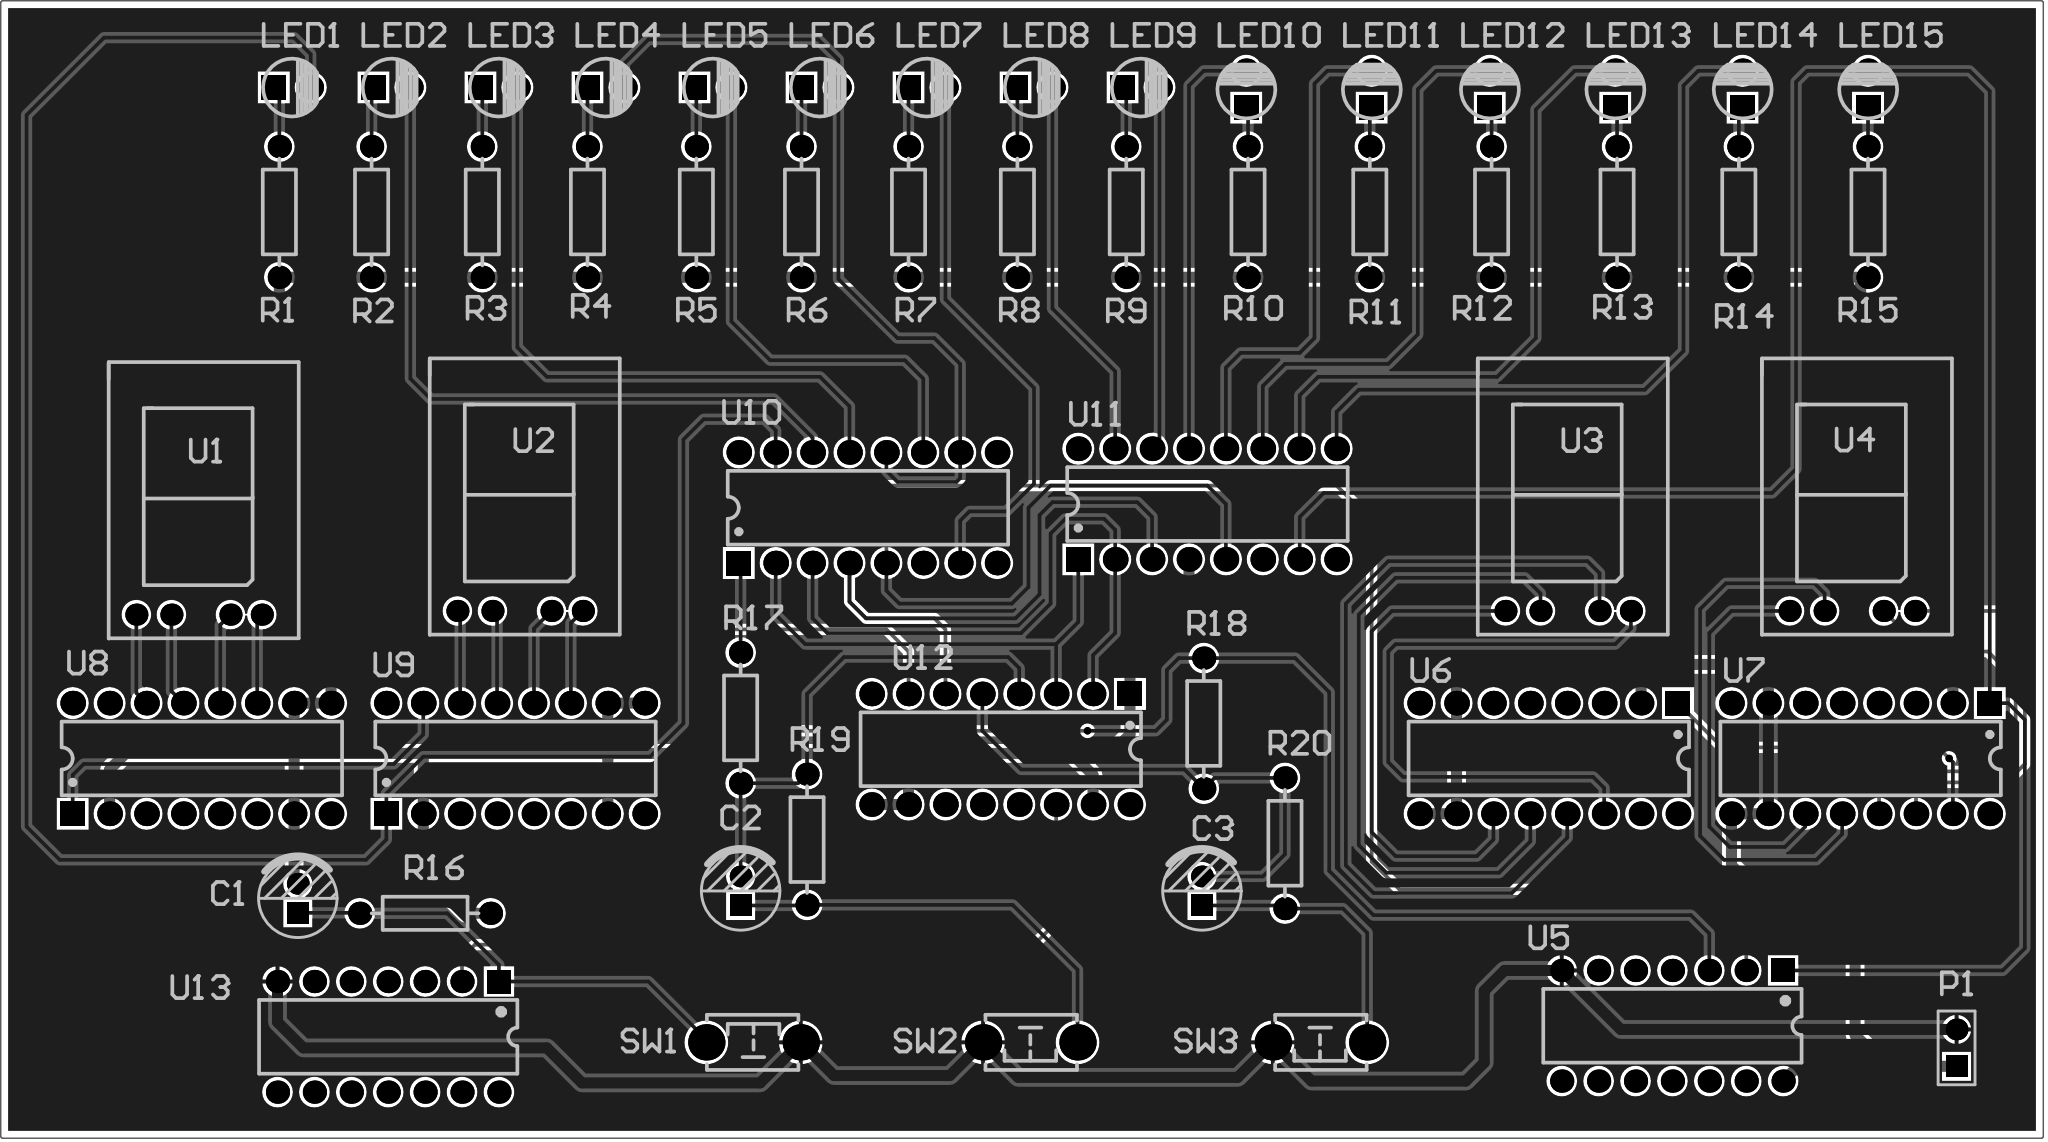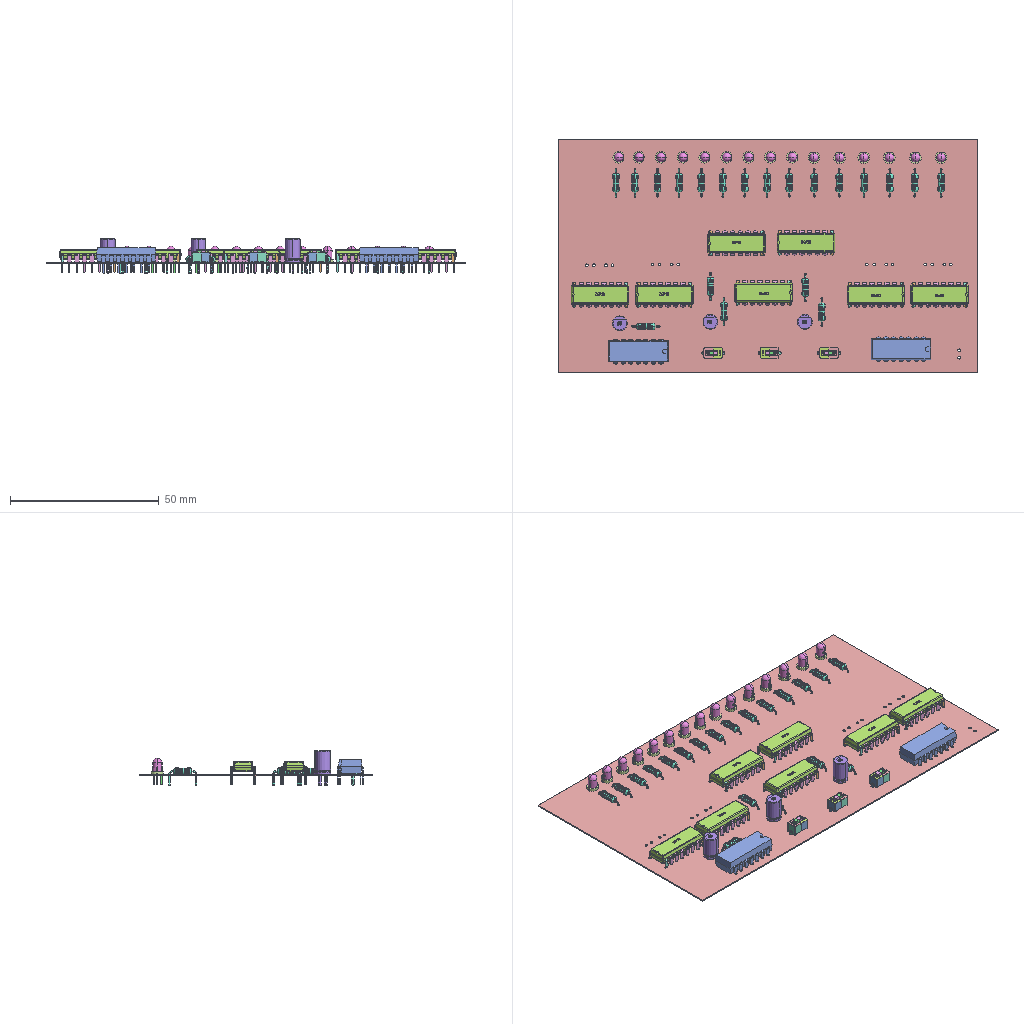Circuit board layout | Altium Designer | box 140.6 x 78.4 x 11.5 mm
Layer stack:
# Altium Designer layer stack of  (unit mm; dielectric type: 0 none, 1 core, 2 prepreg, 3 surface material)
index,name,kind,layer,copper_thickness_mm,dielectric_type,dielectric_thickness_mm,dielectric_material,dielectric_constant
0,Top Paste,other,,,,,,
1,Top Overlay,other,,,,,,
2,Top Solder,dielectric,,,3,0.0102,Solder Resist,3.5
3,Top Layer,copper,Top Layer,0.0356,,,,
4,Dielectric 1,dielectric,,,0,0.32,FR-4,4.8
5,Bottom Layer,copper,Bottom Layer,0.0356,,,,
6,Bottom Solder,dielectric,,,3,0.0102,Solder Resist,3.5
7,Bottom Overlay,other,,,,,,
8,Bottom Paste,other,,,,,,
# drill layer pairs: low layer,high layer
drill_pair,Top Layer,Bottom Layer
Part placement:
Designator,Comment,Layer,Footprint,Center-X(mm),Center-Y(mm),Rotation
U13,SN74LS04D,TopLayer,DIP14,55.118,48.768,270
U12,SN74LS193D,TopLayer,DIP16,97.282,68.58,270
SW3,3x6x5,TopLayer,TSW_DIP-3*6*4.3,119.253,48.387,180
SW2,3x6x5,TopLayer,TSW_DIP-3*6*4.3,99.314,48.387,180
SW1,3x6x5,TopLayer,TSW_DIP-3*6*4.3,80.264,48.387,360
C2,Cap,TopLayer,CS_2.0*5*8_-_C,79.375,58.817,270
C3,Cap,TopLayer,CS_2.0*5*8_-_C,111.125,58.817,270
C1,Cap,TopLayer,CS_2.0*5*8_-_C,48.895,58.309,270
LED1,LED1,TopLayer,LED_3MM-B,48.514,114.173,0
LED2,LED2,TopLayer,LED_3MM-B,55.372,114.173,0
LED3,LED3,TopLayer,LED_3MM-B,62.738,114.173,0
LED4,LED4,TopLayer,LED_3MM-B,70.104,114.173,0
LED5,LED1,TopLayer,LED_3MM-B,77.47,114.173,0
LED6,LED1,TopLayer,LED_3MM-B,84.836,114.173,0
LED7,LED1,TopLayer,LED_3MM-B,92.202,114.173,0
LED8,LED1,TopLayer,LED_3MM-B,99.568,114.173,0
LED9,LED1,TopLayer,LED_3MM-B,106.934,114.173,0
LED10,LED1,TopLayer,LED_3MM-B,114.173,114.046,90
LED11,LED1,TopLayer,LED_3MM-B,122.809,114.046,90
LED12,LED1,TopLayer,LED_3MM-B,130.937,114.046,90
LED13,LED1,TopLayer,LED_3MM-B,139.573,114.046,90
LED14,LED1,TopLayer,LED_3MM-B,148.336,114.046,90
LED15,LED1,TopLayer,LED_3MM-B,156.972,114.046,90
R1,,TopLayer,RS_1/4W,47.625,105.592,270
R2,Res1,TopLayer,RS_1/4W,53.975,105.592,270
R3,Res1,TopLayer,RS_1/4W,61.595,105.592,270
R4,Res1,TopLayer,RS_1/4W,68.834,105.592,270
R5,Res1,TopLayer,RS_1/4W,76.327,105.592,270
R6,Res1,TopLayer,RS_1/4W,83.566,105.592,270
R7,Res1,TopLayer,RS_1/4W,90.932,105.592,270
R8,Res1,TopLayer,RS_1/4W,98.425,105.592,270
R9,Res1,TopLayer,RS_1/4W,105.918,105.592,270
R10,Res1,TopLayer,RS_1/4W,114.3,105.592,270
R11,Res1,TopLayer,RS_1/4W,122.682,105.592,270
R12,Res1,TopLayer,RS_1/4W,131.064,105.592,270
R13,Res1,TopLayer,RS_1/4W,139.7,105.592,270
R14,Res1,TopLayer,RS_1/4W,148.082,105.592,270
R15,Res1,TopLayer,RS_1/4W,156.972,105.592,270
R17,Res1,TopLayer,RS_1/4W,79.375,70.739,90
R18,Res1,TopLayer,RS_1/4W,111.252,70.358,90
R19,Res1,TopLayer,RS_1/4W,83.947,62.357,90
R20,,TopLayer,RS_1/4W,116.84,62.103,90
R16,10k,TopLayer,RS_1/4W,57.658,57.277,360
U1,LCD1,TopLayer,DCD-HEX,42.1,77.851,360
U2,LCD1,TopLayer,DCD-HEX,64.198,78.105,0
U3,LCD1,TopLayer,DCD-HEX,136.334,78.105,0
U4,LCD1,TopLayer,DCD-HEX,155.893,78.105,0
U6,SN74LS160AD,TopLayer,DIP16,135.001,67.945,270
U7,SN74LS160AD,TopLayer,DIP16,156.464,67.945,270
U8,SN74LS160AD,TopLayer,DIP16,42.291,67.945,90
U9,SN74LS160AD,TopLayer,DIP16,63.881,67.945,90
U10,SN74LS138D,TopLayer,DIP16,88.138,85.217,90
U11,SN74LS138D,TopLayer,DIP16,111.506,85.471,90
U5,SN74LS08D,TopLayer,DIP14,143.51,49.53,270
P1,Header 2,TopLayer,HDR1X2,163.068,48.006,90
Pad and via stacks:
# Altium Designer via and pad stacks of  (unit mm). Each distinct definition once, with the count of objects using it.
# via: kind,start_layer,end_layer,hole_mm,diameter_mm,mode(0 simple;1 top-mid-bottom;2 full stack),diameter_per_layer,count,example_net
# pad: kind,layer,hole_mm,hole_type(0 round;1 square;2 slot),plating,top_size,top_shape(1 round;2 rect;3 octagon;9 rounded rect),mid_size,bottom_size,mode,footprint,size_per_layer,count,example
pad,Multi-Layer,0.8,0,plated,1.7x1.7,1,1.7x1.7,1.7x1.7,0,DIP16,,105,U12.16
pad,Multi-Layer,0.8,0,plated,1.7x1.7,2,1.7x1.7,1.7x1.7,0,DIP16,,7,U12.1
pad,Multi-Layer,0.8128,0,plated,1.6x1.6,1,1.6x1.6,1.6x1.6,0,DIP14,,26,U13.14
pad,Multi-Layer,0.8128,0,plated,1.6x1.6,2,1.6x1.6,1.6x1.6,0,DIP14,,2,U13.1
pad,Multi-Layer,1.2,0,plated,2.5x2.5,1,2.5x2.5,2.5x2.5,0,TSW DIP-3*6*4.3,,6,SW1.2
pad,Multi-Layer,0.9144,0,plated,1.524x1.524,1,1.524x1.524,1.524x1.524,0,DCD-HEX,,16,U4.1
pad,Multi-Layer,0.8,0,plated,1.5x1.5,1,1.5x1.5,1.5x1.5,0,CS 2.0*5*8 - C,,3,C3.2
pad,Multi-Layer,0.8,0,plated,1.5x1.5,2,1.5x1.5,1.5x1.5,0,CS 2.0*5*8 - C,,3,C3.1
pad,Multi-Layer,0.6,0,plated,1.6x1.6,1,1.6x1.6,1.6x1.6,0,RS 1/4W,,40,R19.1
pad,Multi-Layer,0.9,0,plated,1.7x1.7,1,1.7x1.7,1.7x1.7,0,LED 3MM-B,,15,LED1.2
pad,Multi-Layer,0.9,0,plated,1.7x1.7,2,1.7x1.7,1.7x1.7,0,LED 3MM-B,,15,LED1.1
pad,Multi-Layer,0.9,0,plated,1.5x1.5,1,1.5x1.5,1.5x1.5,0,HDR1X2,,1,P1.2
pad,Multi-Layer,0.9,0,plated,1.5x1.5,2,1.5x1.5,1.5x1.5,0,HDR1X2,,1,P1.1
via,Top Layer,Bottom Layer,0.254,0.508,0,,2,NetR17_2
Copper pours:
name,layer,net,type(0 solid;1 hatched;2 none)
D,Bottom Layer,GND,0
D,Top Layer,GND,0
Design rules, without the lines most boards share:
# Altium Designer design rules of  (exported by Altium Designer, unit mm)
# columns: name | kind | enabled | priority | scope1 | scope2 | descriptor | typed fields (field=value)
Clearance | 0 | enabled | 1 | All | All | Clearance Constraint (Gap=0.254mm) (All),(All) | gap=0.254
PlaneConnect | 6 | enabled | 1 | All | All | Power Plane Connect Rule(Relief Connect )(Expansion=0.508mm) (Conductor Width=0.254mm) (Air Gap=0.254mm) (Entries=4) (All) | relief_conductor_width=0.254 relief_entries=4 relief_expansion=0.508
PlaneClearance | 12 | enabled | 1 | All | All | Power Plane Clearance (Clearance =0.508mm) (All) | clearance=0.508
PolygonConnect | 20 | enabled | 1 | All | All | Polygon Connect Rule(Relief Connect )(Conductor Width=0.254mm) (Relief Angle=90 Angle) (Entries=4) (Air Gap Width=0.254mm) (All),(All) | connect_style(0=relief,1=direct,2=none)=0 relief_conductor_width=0.254 relief_entries=4
Width | 2 | enabled | 1 | All | All | Width Constraint (Min=0.254mm) (Max=0.762mm) (Preferred=0.254mm) (All) |
RoutingCorners | 10 | enabled | 1 | All | All | Routing Corners (Style=45-Degree) (Min Setback=2.54mm) (Max Setback=2.54mm) (All) |
RoutingVias | 11 | enabled | 1 | All | All | Routing Via (MinHoleWidth=0.711mm) (MaxHoleWidth=0.711mm) (PreferredHoleWidth=0.711mm) (MinWidth=1.27mm) (MaxWidth=1.27mm) (PreferedWidth=1.27mm) (All) | via_min_hole=0.7112 via_max_hole=0.7112 via_preferred_diameter=1.27 via_preferred_hole=0.7112
PasteMaskExpansion | 14 | enabled | 1 | All | All | Paste Mask Expansion (Expansion =0mm) (All) | expansion=0
SolderMaskExpansion | 13 | enabled | 1 | All | All | Solder Mask Expansion (Expansion =0.102mm) (All) | expansion=0.1016
ComponentClearance | 24 | enabled | 1 | All | All | Component Clearance Constraint ( Horizontal Gap = 0.254mm, Vertical Gap = 0.254mm ) (All),(All)  | gap=0.254
Height | 50 | enabled | 1 | All | All | Height Constraint (Min=0mm) (Max=25.4mm) (Prefered=12.7mm) (All) | min_height=0 max_height=25.4
HoleSize | 42 | enabled | 1 | All | All | Hole Size Constraint (Min=0.025mm) (Max=2.54mm) (All) |
DiffPairsRouting | 51 | enabled | 1 | All | All | Differential Pairs Uncoupled Length using the Gap Constraints (Min=0.254mm) (Max=0.254mm) (Prefered=0.254mm)  and Width Constraints (Min=0.381mm) (Max=0.381mm) (Prefered=0.381mm) (All) |
HoleToHoleClearance | 52 | enabled | 1 | All | All | Hole To Hole Clearance (Gap=0.254mm) (All),(All) | gap=0.254
MinimumSolderMaskSliver | 53 | enabled | 1 | All | All | Minimum Solder Mask Sliver (Gap=0mm) (All),(All) |
SilkToSolderMaskClearance | 54 | enabled | 1 | IsPad | All | Silk To Solder Mask (Clearance=0mm) (IsPad),(All) |
SilkToSilkClearance | 55 | enabled | 1 | All | All | Silk to Silk (Clearance=0mm) (All),(All) |
NetAntennae | 56 | enabled | 1 | All | All | Net Antennae (Tolerance=0mm) (All) |